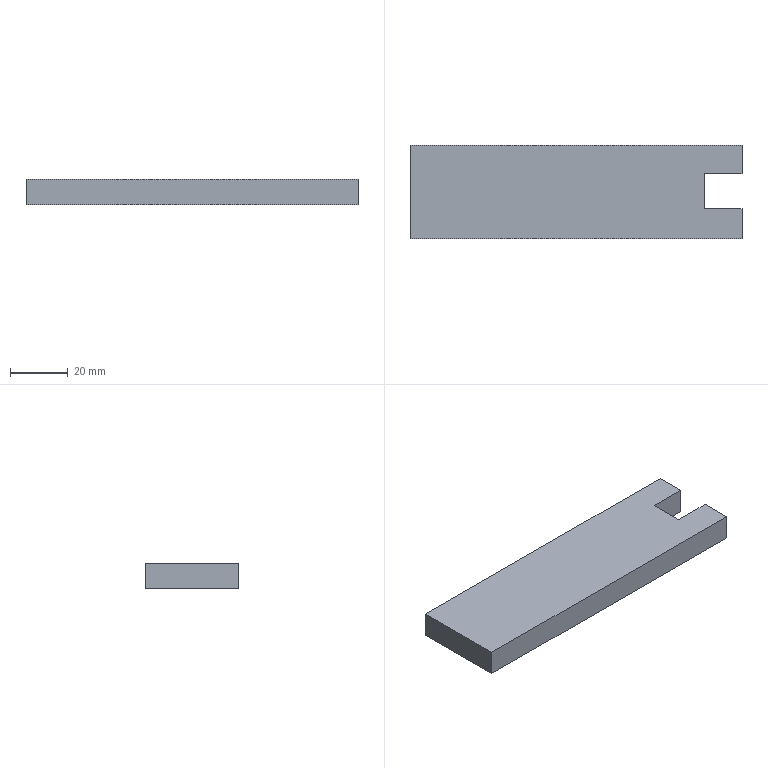Part | STEP file | BU-D02#180c | 1 solid | 30 faces | box 115 x 32.5 x 9 mm | volume 31043 mm3 | plane 14 | cylinder 12 | cone 4 | commonest cylinder face diameters 3.3 x4 4.5 x4 8 x4